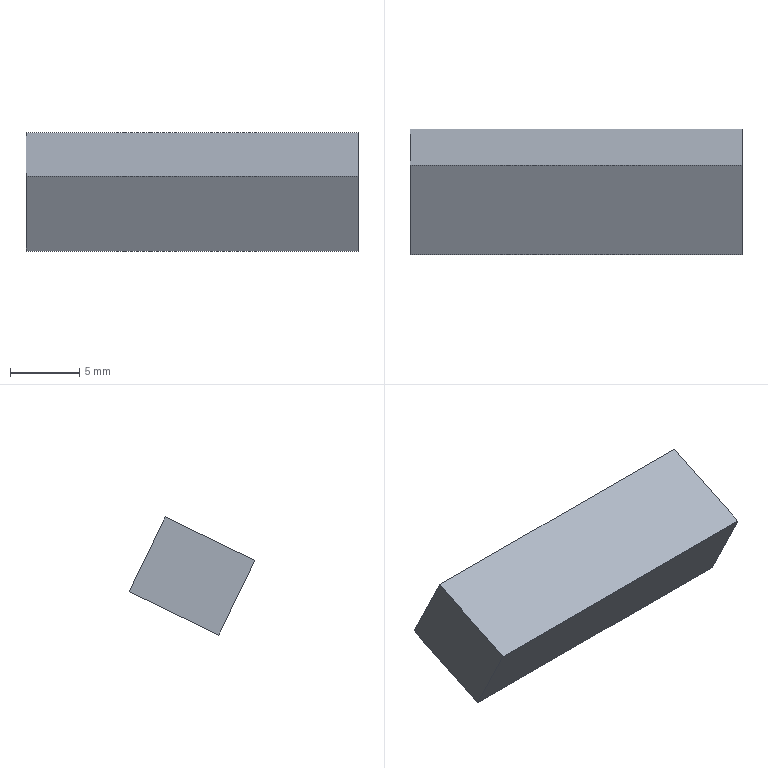Part | NX | 1 solid | 6 faces | box 24 x 9.093 x 8.534 mm | volume 1037 mm3 | plane 6
STEP:
#1=CARTESIAN_POINT('',(4.494,-554.691,2407.049));
#2=VERTEX_POINT('',#1);
#3=CARTESIAN_POINT('',(4.494,-548.207,2410.179));
#4=VERTEX_POINT('',#3);
#5=CARTESIAN_POINT('',(4.494,-548.207,2410.179));
#6=DIRECTION('',(0.,0.9005,0.4348));
#7=VECTOR('',#6,1.);
#8=LINE('',#5,#7);
#9=EDGE_CURVE('',#2,#4,#8,.T.);
#10=ORIENTED_EDGE('',*,*,#9,.F.);
#11=CARTESIAN_POINT('',(28.494,-554.691,2407.049));
#12=VERTEX_POINT('',#11);
#13=CARTESIAN_POINT('',(28.494,-554.691,2407.049));
#14=DIRECTION('',(-1.,0.,0.));
#15=VECTOR('',#14,1.);
#16=LINE('',#13,#15);
#17=EDGE_CURVE('',#12,#2,#16,.T.);
#18=ORIENTED_EDGE('',*,*,#17,.F.);
#19=CARTESIAN_POINT('',(28.494,-548.207,2410.179));
#20=VERTEX_POINT('',#19);
#21=CARTESIAN_POINT('',(28.494,-548.207,2410.179));
#22=DIRECTION('',(0.,0.9005,0.4348));
#23=VECTOR('',#22,1.);
#24=LINE('',#21,#23);
#25=EDGE_CURVE('',#12,#20,#24,.T.);
#26=ORIENTED_EDGE('',*,*,#25,.T.);
#27=CARTESIAN_POINT('',(28.494,-548.207,2410.179));
#28=DIRECTION('',(-1.,0.,0.));
#29=VECTOR('',#28,1.);
#30=LINE('',#27,#29);
#31=EDGE_CURVE('',#20,#4,#30,.T.);
#32=ORIENTED_EDGE('',*,*,#31,.T.);
#33=EDGE_LOOP('',(#10,#18,#26,#32));
#34=FACE_OUTER_BOUND('',#33,.T.);
#35=CARTESIAN_POINT('',(28.494,-548.207,2410.179));
#36=DIRECTION('',(0.,-0.4348,0.9005));
#37=DIRECTION('',(-1.,0.,0.));
#38=AXIS2_PLACEMENT_3D('',#35,#36,#37);
#39=PLANE('',#38);
#40=ADVANCED_FACE('',(#34),#39,.T.);
#41=CARTESIAN_POINT('',(4.494,-552.082,2401.645));
#42=VERTEX_POINT('',#41);
#43=CARTESIAN_POINT('',(4.494,-554.691,2407.049));
#44=DIRECTION('',(0.,-0.4348,0.9005));
#45=VECTOR('',#44,1.);
#46=LINE('',#43,#45);
#47=EDGE_CURVE('',#42,#2,#46,.T.);
#48=ORIENTED_EDGE('',*,*,#47,.F.);
#49=CARTESIAN_POINT('',(28.494,-552.082,2401.645));
#50=VERTEX_POINT('',#49);
#51=CARTESIAN_POINT('',(28.494,-552.082,2401.645));
#52=DIRECTION('',(-1.,0.,0.));
#53=VECTOR('',#52,1.);
#54=LINE('',#51,#53);
#55=EDGE_CURVE('',#50,#42,#54,.T.);
#56=ORIENTED_EDGE('',*,*,#55,.F.);
#57=CARTESIAN_POINT('',(28.494,-554.691,2407.049));
#58=DIRECTION('',(0.,-0.4348,0.9005));
#59=VECTOR('',#58,1.);
#60=LINE('',#57,#59);
#61=EDGE_CURVE('',#50,#12,#60,.T.);
#62=ORIENTED_EDGE('',*,*,#61,.T.);
#63=ORIENTED_EDGE('',*,*,#17,.T.);
#64=EDGE_LOOP('',(#48,#56,#62,#63));
#65=FACE_OUTER_BOUND('',#64,.T.);
#66=CARTESIAN_POINT('',(28.494,-554.691,2407.049));
#67=DIRECTION('',(0.,-0.9005,-0.4348));
#68=DIRECTION('',(0.,0.4348,-0.9005));
#69=AXIS2_PLACEMENT_3D('',#66,#67,#68);
#70=PLANE('',#69);
#71=ADVANCED_FACE('',(#65),#70,.T.);
#72=CARTESIAN_POINT('',(4.494,-545.598,2404.776));
#73=VERTEX_POINT('',#72);
#74=CARTESIAN_POINT('',(4.494,-545.598,2404.776));
#75=DIRECTION('',(0.,-0.9005,-0.4348));
#76=VECTOR('',#75,1.);
#77=LINE('',#74,#76);
#78=EDGE_CURVE('',#73,#42,#77,.T.);
#79=ORIENTED_EDGE('',*,*,#78,.F.);
#80=CARTESIAN_POINT('',(28.494,-545.598,2404.776));
#81=VERTEX_POINT('',#80);
#82=CARTESIAN_POINT('',(28.494,-545.598,2404.776));
#83=DIRECTION('',(-1.,0.,0.));
#84=VECTOR('',#83,1.);
#85=LINE('',#82,#84);
#86=EDGE_CURVE('',#81,#73,#85,.T.);
#87=ORIENTED_EDGE('',*,*,#86,.F.);
#88=CARTESIAN_POINT('',(28.494,-545.598,2404.776));
#89=DIRECTION('',(0.,-0.9005,-0.4348));
#90=VECTOR('',#89,1.);
#91=LINE('',#88,#90);
#92=EDGE_CURVE('',#81,#50,#91,.T.);
#93=ORIENTED_EDGE('',*,*,#92,.T.);
#94=ORIENTED_EDGE('',*,*,#55,.T.);
#95=EDGE_LOOP('',(#79,#87,#93,#94));
#96=FACE_OUTER_BOUND('',#95,.T.);
#97=CARTESIAN_POINT('',(28.494,-545.598,2404.776));
#98=DIRECTION('',(0.,0.4348,-0.9005));
#99=DIRECTION('',(1.,0.,0.));
#100=AXIS2_PLACEMENT_3D('',#97,#98,#99);
#101=PLANE('',#100);
#102=ADVANCED_FACE('',(#96),#101,.T.);
#103=CARTESIAN_POINT('',(4.494,-548.207,2410.179));
#104=DIRECTION('',(0.,0.4348,-0.9005));
#105=VECTOR('',#104,1.);
#106=LINE('',#103,#105);
#107=EDGE_CURVE('',#4,#73,#106,.T.);
#108=ORIENTED_EDGE('',*,*,#107,.F.);
#109=ORIENTED_EDGE('',*,*,#31,.F.);
#110=CARTESIAN_POINT('',(28.494,-548.207,2410.179));
#111=DIRECTION('',(0.,0.4348,-0.9005));
#112=VECTOR('',#111,1.);
#113=LINE('',#110,#112);
#114=EDGE_CURVE('',#20,#81,#113,.T.);
#115=ORIENTED_EDGE('',*,*,#114,.T.);
#116=ORIENTED_EDGE('',*,*,#86,.T.);
#117=EDGE_LOOP('',(#108,#109,#115,#116));
#118=FACE_OUTER_BOUND('',#117,.T.);
#119=CARTESIAN_POINT('',(28.494,-548.207,2410.179));
#120=DIRECTION('',(0.,0.9005,0.4348));
#121=DIRECTION('',(0.,-0.4348,0.9005));
#122=AXIS2_PLACEMENT_3D('',#119,#120,#121);
#123=PLANE('',#122);
#124=ADVANCED_FACE('',(#118),#123,.T.);
#125=ORIENTED_EDGE('',*,*,#25,.F.);
#126=ORIENTED_EDGE('',*,*,#61,.F.);
#127=ORIENTED_EDGE('',*,*,#92,.F.);
#128=ORIENTED_EDGE('',*,*,#114,.F.);
#129=EDGE_LOOP('',(#125,#126,#127,#128));
#130=FACE_OUTER_BOUND('',#129,.T.);
#131=CARTESIAN_POINT('',(28.494,-554.691,2407.049));
#132=DIRECTION('',(1.,0.,0.));
#133=DIRECTION('',(0.,-0.4348,0.9005));
#134=AXIS2_PLACEMENT_3D('',#131,#132,#133);
#135=PLANE('',#134);
#136=ADVANCED_FACE('',(#130),#135,.T.);
#137=ORIENTED_EDGE('',*,*,#9,.T.);
#138=ORIENTED_EDGE('',*,*,#107,.T.);
#139=ORIENTED_EDGE('',*,*,#78,.T.);
#140=ORIENTED_EDGE('',*,*,#47,.T.);
#141=EDGE_LOOP('',(#137,#138,#139,#140));
#142=FACE_OUTER_BOUND('',#141,.T.);
#143=CARTESIAN_POINT('',(4.494,-554.691,2407.049));
#144=DIRECTION('',(1.,0.,0.));
#145=DIRECTION('',(0.,-0.4348,0.9005));
#146=AXIS2_PLACEMENT_3D('',#143,#144,#145);
#147=PLANE('',#146);
#148=ADVANCED_FACE('',(#142),#147,.F.);
#149=CLOSED_SHELL('',(#40,#71,#102,#124,#136,#148));
#150=MANIFOLD_SOLID_BREP('',#149);
#151=(LENGTH_UNIT()NAMED_UNIT(*)SI_UNIT(.MILLI.,.METRE.));
#152=UNCERTAINTY_MEASURE_WITH_UNIT(LENGTH_MEASURE(0.00002),#151,'','');
#153=(NAMED_UNIT(*)PLANE_ANGLE_UNIT()SI_UNIT($,.RADIAN.));
#154=PLANE_ANGLE_MEASURE_WITH_UNIT(PLANE_ANGLE_MEASURE(0.01745),#153);
#155=DIMENSIONAL_EXPONENTS(0.,0.,0.,0.,0.,0.,0.);
#156=(CONVERSION_BASED_UNIT('DEGREE',#154)NAMED_UNIT(#155)PLANE_ANGLE_UNIT());
#157=(NAMED_UNIT(*)SI_UNIT($,.STERADIAN.)SOLID_ANGLE_UNIT());
#158=(GEOMETRIC_REPRESENTATION_CONTEXT(3)GLOBAL_UNCERTAINTY_ASSIGNED_CONTEXT((#152))GLOBAL_UNIT_ASSIGNED_CONTEXT((#151,#156,#157))REPRESENTATION_CONTEXT('',''));
#159=ADVANCED_BREP_SHAPE_REPRESENTATION('',(#150),#158);